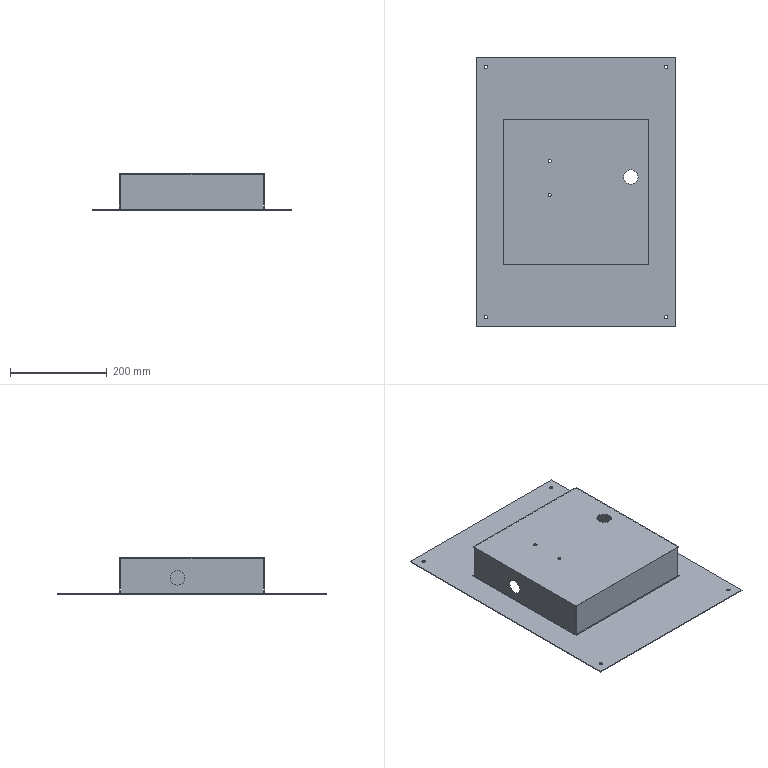Part | STEP file | 09-28 closing plate E (Default) | 1 solid | 56 faces | box 413 x 558 x 75 mm | volume 472470 mm3 | cylinder 24 | plane 24 | spline 8 | commonest cylinder face diameters 7 x8 1.473 x4 4.473 x4 6.5 x4 30 x4